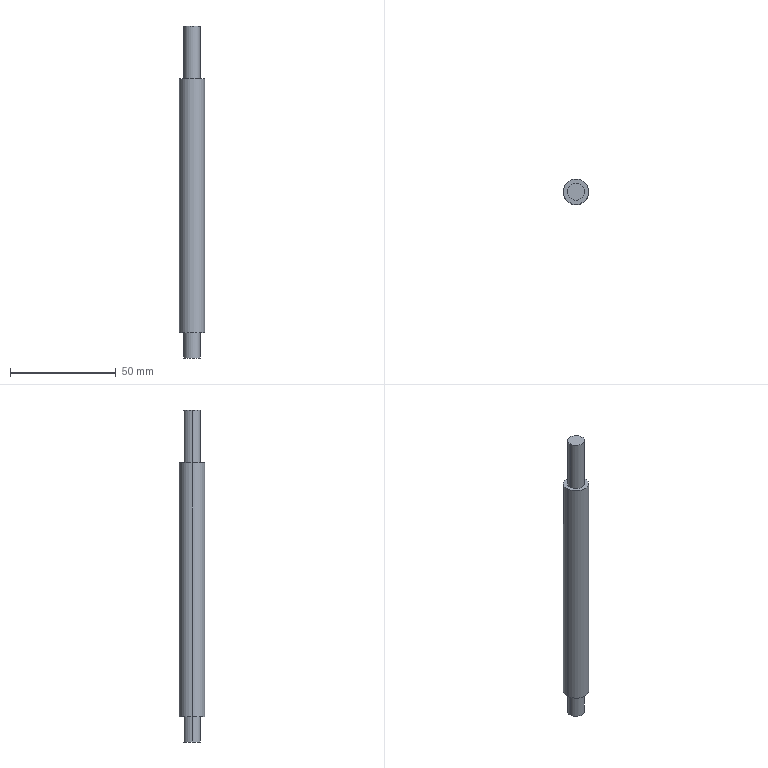Part | SolidWorks | features ICE 2, Extrusion 1 | 1 solid | 10 faces | box 12 x 12 x 157 mm | volume 15432 mm3 | cylinder 6 | plane 4 | commonest cylinder face diameters 8 x4 12 x2
STEP:
#1=CARTESIAN_POINT('',(4.,0.,145.));
#2=VERTEX_POINT('',#1);
#3=CARTESIAN_POINT('',(-4.,0.,145.));
#4=VERTEX_POINT('',#3);
#5=CARTESIAN_POINT('',(0.,0.,145.));
#6=DIRECTION('',(0.,0.,1.));
#7=DIRECTION('',(1.,0.,0.));
#8=AXIS2_PLACEMENT_3D('',#5,#6,#7);
#9=CIRCLE('',#8,4.);
#10=EDGE_CURVE('',#2,#4,#9,.T.);
#11=ORIENTED_EDGE('',*,*,#10,.F.);
#12=CARTESIAN_POINT('',(4.,0.,120.));
#13=VERTEX_POINT('',#12);
#14=CARTESIAN_POINT('',(4.,0.,145.));
#15=DIRECTION('',(0.,0.,-1.));
#16=VECTOR('',#15,1000.);
#17=LINE('',#14,#16);
#18=EDGE_CURVE('',#2,#13,#17,.T.);
#19=ORIENTED_EDGE('',*,*,#18,.T.);
#20=CARTESIAN_POINT('',(-4.,0.,120.));
#21=VERTEX_POINT('',#20);
#22=CARTESIAN_POINT('',(0.,0.,120.));
#23=DIRECTION('',(0.,0.,1.));
#24=DIRECTION('',(1.,0.,0.));
#25=AXIS2_PLACEMENT_3D('',#22,#23,#24);
#26=CIRCLE('',#25,4.);
#27=EDGE_CURVE('',#13,#21,#26,.T.);
#28=ORIENTED_EDGE('',*,*,#27,.T.);
#29=CARTESIAN_POINT('',(-4.,0.,145.));
#30=DIRECTION('',(0.,0.,-1.));
#31=VECTOR('',#30,1000.);
#32=LINE('',#29,#31);
#33=EDGE_CURVE('',#4,#21,#32,.T.);
#34=ORIENTED_EDGE('',*,*,#33,.F.);
#35=EDGE_LOOP('',(#11,#19,#28,#34));
#36=FACE_OUTER_BOUND('',#35,.T.);
#37=CARTESIAN_POINT('',(0.,0.,145.));
#38=DIRECTION('',(0.,0.,-1.));
#39=DIRECTION('',(-1.,0.,0.));
#40=AXIS2_PLACEMENT_3D('',#37,#38,#39);
#41=CYLINDRICAL_SURFACE('',#40,4.);
#42=ADVANCED_FACE('',(#36),#41,.T.);
#43=CARTESIAN_POINT('',(-4.,0.,-12.));
#44=VERTEX_POINT('',#43);
#45=CARTESIAN_POINT('',(4.,0.,-12.));
#46=VERTEX_POINT('',#45);
#47=CARTESIAN_POINT('',(0.,0.,-12.));
#48=DIRECTION('',(0.,0.,-1.));
#49=DIRECTION('',(-1.,0.,0.));
#50=AXIS2_PLACEMENT_3D('',#47,#48,#49);
#51=CIRCLE('',#50,4.);
#52=EDGE_CURVE('',#44,#46,#51,.T.);
#53=ORIENTED_EDGE('',*,*,#52,.F.);
#54=CARTESIAN_POINT('',(-4.,0.,0.));
#55=VERTEX_POINT('',#54);
#56=CARTESIAN_POINT('',(-4.,0.,-12.));
#57=DIRECTION('',(0.,0.,1.));
#58=VECTOR('',#57,1000.);
#59=LINE('',#56,#58);
#60=EDGE_CURVE('',#44,#55,#59,.T.);
#61=ORIENTED_EDGE('',*,*,#60,.T.);
#62=CARTESIAN_POINT('',(4.,0.,0.));
#63=VERTEX_POINT('',#62);
#64=CARTESIAN_POINT('',(0.,0.,0.));
#65=DIRECTION('',(0.,0.,-1.));
#66=DIRECTION('',(-1.,0.,0.));
#67=AXIS2_PLACEMENT_3D('',#64,#65,#66);
#68=CIRCLE('',#67,4.);
#69=EDGE_CURVE('',#55,#63,#68,.T.);
#70=ORIENTED_EDGE('',*,*,#69,.T.);
#71=CARTESIAN_POINT('',(4.,0.,-12.));
#72=DIRECTION('',(0.,0.,1.));
#73=VECTOR('',#72,1000.);
#74=LINE('',#71,#73);
#75=EDGE_CURVE('',#46,#63,#74,.T.);
#76=ORIENTED_EDGE('',*,*,#75,.F.);
#77=EDGE_LOOP('',(#53,#61,#70,#76));
#78=FACE_OUTER_BOUND('',#77,.T.);
#79=CARTESIAN_POINT('',(0.,0.,-12.));
#80=DIRECTION('',(0.,0.,1.));
#81=DIRECTION('',(1.,0.,0.));
#82=AXIS2_PLACEMENT_3D('',#79,#80,#81);
#83=CYLINDRICAL_SURFACE('',#82,4.);
#84=ADVANCED_FACE('',(#78),#83,.T.);
#85=CARTESIAN_POINT('',(6.,0.,120.));
#86=VERTEX_POINT('',#85);
#87=CARTESIAN_POINT('',(-6.,0.,120.));
#88=VERTEX_POINT('',#87);
#89=CARTESIAN_POINT('',(0.,0.,120.));
#90=DIRECTION('',(0.,0.,1.));
#91=DIRECTION('',(1.,0.,0.));
#92=AXIS2_PLACEMENT_3D('',#89,#90,#91);
#93=CIRCLE('',#92,6.);
#94=EDGE_CURVE('',#86,#88,#93,.T.);
#95=ORIENTED_EDGE('',*,*,#94,.F.);
#96=CARTESIAN_POINT('',(6.,0.,0.));
#97=VERTEX_POINT('',#96);
#98=CARTESIAN_POINT('',(6.,0.,120.));
#99=DIRECTION('',(0.,0.,-1.));
#100=VECTOR('',#99,1000.);
#101=LINE('',#98,#100);
#102=EDGE_CURVE('',#86,#97,#101,.T.);
#103=ORIENTED_EDGE('',*,*,#102,.T.);
#104=CARTESIAN_POINT('',(-6.,0.,0.));
#105=VERTEX_POINT('',#104);
#106=CARTESIAN_POINT('',(0.,0.,0.));
#107=DIRECTION('',(0.,0.,1.));
#108=DIRECTION('',(1.,0.,0.));
#109=AXIS2_PLACEMENT_3D('',#106,#107,#108);
#110=CIRCLE('',#109,6.);
#111=EDGE_CURVE('',#97,#105,#110,.T.);
#112=ORIENTED_EDGE('',*,*,#111,.T.);
#113=CARTESIAN_POINT('',(-6.,0.,120.));
#114=DIRECTION('',(0.,0.,-1.));
#115=VECTOR('',#114,1000.);
#116=LINE('',#113,#115);
#117=EDGE_CURVE('',#88,#105,#116,.T.);
#118=ORIENTED_EDGE('',*,*,#117,.F.);
#119=EDGE_LOOP('',(#95,#103,#112,#118));
#120=FACE_OUTER_BOUND('',#119,.T.);
#121=CARTESIAN_POINT('',(0.,0.,120.));
#122=DIRECTION('',(0.,0.,-1.));
#123=DIRECTION('',(-1.,0.,0.));
#124=AXIS2_PLACEMENT_3D('',#121,#122,#123);
#125=CYLINDRICAL_SURFACE('',#124,6.);
#126=ADVANCED_FACE('',(#120),#125,.T.);
#127=ORIENTED_EDGE('',*,*,#102,.F.);
#128=CARTESIAN_POINT('',(0.,0.,120.));
#129=DIRECTION('',(0.,0.,1.));
#130=DIRECTION('',(1.,0.,0.));
#131=AXIS2_PLACEMENT_3D('',#128,#129,#130);
#132=CIRCLE('',#131,6.);
#133=EDGE_CURVE('',#88,#86,#132,.T.);
#134=ORIENTED_EDGE('',*,*,#133,.F.);
#135=ORIENTED_EDGE('',*,*,#117,.T.);
#136=CARTESIAN_POINT('',(0.,0.,0.));
#137=DIRECTION('',(0.,0.,1.));
#138=DIRECTION('',(1.,0.,0.));
#139=AXIS2_PLACEMENT_3D('',#136,#137,#138);
#140=CIRCLE('',#139,6.);
#141=EDGE_CURVE('',#105,#97,#140,.T.);
#142=ORIENTED_EDGE('',*,*,#141,.T.);
#143=EDGE_LOOP('',(#127,#134,#135,#142));
#144=FACE_OUTER_BOUND('',#143,.T.);
#145=CARTESIAN_POINT('',(0.,0.,120.));
#146=DIRECTION('',(0.,0.,-1.));
#147=DIRECTION('',(-1.,0.,0.));
#148=AXIS2_PLACEMENT_3D('',#145,#146,#147);
#149=CYLINDRICAL_SURFACE('',#148,6.);
#150=ADVANCED_FACE('',(#144),#149,.T.);
#151=CARTESIAN_POINT('',(0.,0.,120.));
#152=DIRECTION('',(0.,0.,1.));
#153=DIRECTION('',(1.,0.,0.));
#154=AXIS2_PLACEMENT_3D('',#151,#152,#153);
#155=CIRCLE('',#154,4.);
#156=EDGE_CURVE('',#21,#13,#155,.T.);
#157=ORIENTED_EDGE('',*,*,#156,.F.);
#158=ORIENTED_EDGE('',*,*,#27,.F.);
#159=EDGE_LOOP('',(#157,#158));
#160=FACE_BOUND('',#159,.T.);
#161=ORIENTED_EDGE('',*,*,#133,.T.);
#162=ORIENTED_EDGE('',*,*,#94,.T.);
#163=EDGE_LOOP('',(#161,#162));
#164=FACE_OUTER_BOUND('',#163,.T.);
#165=CARTESIAN_POINT('',(0.,0.,120.));
#166=DIRECTION('',(0.,0.,1.));
#167=DIRECTION('',(1.,0.,0.));
#168=AXIS2_PLACEMENT_3D('',#165,#166,#167);
#169=PLANE('',#168);
#170=ADVANCED_FACE('',(#160,#164),#169,.T.);
#171=CARTESIAN_POINT('',(0.,0.,0.));
#172=DIRECTION('',(0.,0.,-1.));
#173=DIRECTION('',(-1.,0.,0.));
#174=AXIS2_PLACEMENT_3D('',#171,#172,#173);
#175=CIRCLE('',#174,4.);
#176=EDGE_CURVE('',#63,#55,#175,.T.);
#177=ORIENTED_EDGE('',*,*,#176,.F.);
#178=ORIENTED_EDGE('',*,*,#69,.F.);
#179=EDGE_LOOP('',(#177,#178));
#180=FACE_BOUND('',#179,.T.);
#181=ORIENTED_EDGE('',*,*,#141,.F.);
#182=ORIENTED_EDGE('',*,*,#111,.F.);
#183=EDGE_LOOP('',(#181,#182));
#184=FACE_OUTER_BOUND('',#183,.T.);
#185=CARTESIAN_POINT('',(0.,0.,0.));
#186=DIRECTION('',(0.,0.,1.));
#187=DIRECTION('',(1.,0.,0.));
#188=AXIS2_PLACEMENT_3D('',#185,#186,#187);
#189=PLANE('',#188);
#190=ADVANCED_FACE('',(#180,#184),#189,.F.);
#191=ORIENTED_EDGE('',*,*,#60,.F.);
#192=CARTESIAN_POINT('',(0.,0.,-12.));
#193=DIRECTION('',(0.,0.,-1.));
#194=DIRECTION('',(-1.,0.,0.));
#195=AXIS2_PLACEMENT_3D('',#192,#193,#194);
#196=CIRCLE('',#195,4.);
#197=EDGE_CURVE('',#46,#44,#196,.T.);
#198=ORIENTED_EDGE('',*,*,#197,.F.);
#199=ORIENTED_EDGE('',*,*,#75,.T.);
#200=ORIENTED_EDGE('',*,*,#176,.T.);
#201=EDGE_LOOP('',(#191,#198,#199,#200));
#202=FACE_OUTER_BOUND('',#201,.T.);
#203=CARTESIAN_POINT('',(0.,0.,-12.));
#204=DIRECTION('',(0.,0.,1.));
#205=DIRECTION('',(1.,0.,0.));
#206=AXIS2_PLACEMENT_3D('',#203,#204,#205);
#207=CYLINDRICAL_SURFACE('',#206,4.);
#208=ADVANCED_FACE('',(#202),#207,.T.);
#209=ORIENTED_EDGE('',*,*,#197,.T.);
#210=ORIENTED_EDGE('',*,*,#52,.T.);
#211=EDGE_LOOP('',(#209,#210));
#212=FACE_OUTER_BOUND('',#211,.T.);
#213=CARTESIAN_POINT('',(0.,0.,-12.));
#214=DIRECTION('',(0.,0.,-1.));
#215=DIRECTION('',(-1.,0.,0.));
#216=AXIS2_PLACEMENT_3D('',#213,#214,#215);
#217=PLANE('',#216);
#218=ADVANCED_FACE('',(#212),#217,.T.);
#219=ORIENTED_EDGE('',*,*,#18,.F.);
#220=CARTESIAN_POINT('',(0.,0.,145.));
#221=DIRECTION('',(0.,0.,1.));
#222=DIRECTION('',(1.,0.,0.));
#223=AXIS2_PLACEMENT_3D('',#220,#221,#222);
#224=CIRCLE('',#223,4.);
#225=EDGE_CURVE('',#4,#2,#224,.T.);
#226=ORIENTED_EDGE('',*,*,#225,.F.);
#227=ORIENTED_EDGE('',*,*,#33,.T.);
#228=ORIENTED_EDGE('',*,*,#156,.T.);
#229=EDGE_LOOP('',(#219,#226,#227,#228));
#230=FACE_OUTER_BOUND('',#229,.T.);
#231=CARTESIAN_POINT('',(0.,0.,145.));
#232=DIRECTION('',(0.,0.,-1.));
#233=DIRECTION('',(-1.,0.,0.));
#234=AXIS2_PLACEMENT_3D('',#231,#232,#233);
#235=CYLINDRICAL_SURFACE('',#234,4.);
#236=ADVANCED_FACE('',(#230),#235,.T.);
#237=ORIENTED_EDGE('',*,*,#225,.T.);
#238=ORIENTED_EDGE('',*,*,#10,.T.);
#239=EDGE_LOOP('',(#237,#238));
#240=FACE_OUTER_BOUND('',#239,.T.);
#241=CARTESIAN_POINT('',(0.,0.,145.));
#242=DIRECTION('',(0.,0.,1.));
#243=DIRECTION('',(1.,0.,0.));
#244=AXIS2_PLACEMENT_3D('',#241,#242,#243);
#245=PLANE('',#244);
#246=ADVANCED_FACE('',(#240),#245,.T.);
#247=CLOSED_SHELL('',(#42,#84,#126,#150,#170,#190,#208,#218,#236,#246));
#248=MANIFOLD_SOLID_BREP('',#247);
#249=CARTESIAN_POINT('',(0.,0.,0.));
#250=DIRECTION('',(0.,0.,1.));
#251=DIRECTION('',(1.,0.,0.));
#252=AXIS2_PLACEMENT_3D('',#249,#250,#251);
#253=(LENGTH_UNIT()NAMED_UNIT(*)SI_UNIT(.MILLI.,.METRE.));
#254=UNCERTAINTY_MEASURE_WITH_UNIT(LENGTH_MEASURE(0.00001),#253,'','');
#255=(NAMED_UNIT(*)PLANE_ANGLE_UNIT()SI_UNIT($,.RADIAN.));
#256=(NAMED_UNIT(*)SI_UNIT($,.STERADIAN.)SOLID_ANGLE_UNIT());
#257=(GEOMETRIC_REPRESENTATION_CONTEXT(3)GLOBAL_UNCERTAINTY_ASSIGNED_CONTEXT((#254))GLOBAL_UNIT_ASSIGNED_CONTEXT((#253,#255,#256))REPRESENTATION_CONTEXT('',''));
#258=ADVANCED_BREP_SHAPE_REPRESENTATION('',(#248,#252),#257);